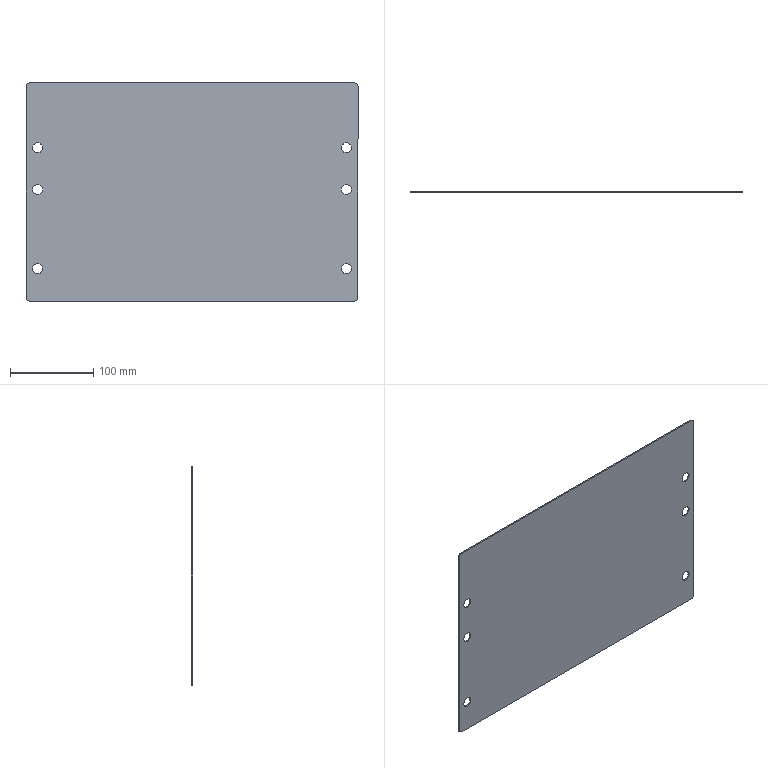Part | SolidWorks | features Fillet 1, FlatPattern 1, HoleWzd 1, SMBaseFlange 1, SheetMetal 1 | 1 solid | 22 faces | box 398 x 1.5 x 262 mm | volume 155364 mm3 | cylinder 16 | plane 6 | commonest cylinder face diameters 12 x12 10 x4
STEP:
#1=CARTESIAN_POINT('',(-185.,-1.5,-3.));
#2=VERTEX_POINT('',#1);
#3=CARTESIAN_POINT('',(-185.,-1.5,9.));
#4=VERTEX_POINT('',#3);
#5=CARTESIAN_POINT('',(-185.,-1.5,3.));
#6=DIRECTION('',(0.,1.,0.));
#7=DIRECTION('',(0.,0.,1.));
#8=AXIS2_PLACEMENT_3D('',#5,#6,#7);
#9=CIRCLE('',#8,6.);
#10=EDGE_CURVE('',#2,#4,#9,.T.);
#11=ORIENTED_EDGE('',*,*,#10,.F.);
#12=CARTESIAN_POINT('',(-185.,0.,-3.));
#13=VERTEX_POINT('',#12);
#14=CARTESIAN_POINT('',(-185.,0.,-3.));
#15=DIRECTION('',(0.,1.,0.));
#16=VECTOR('',#15,1000.);
#17=LINE('',#14,#16);
#18=EDGE_CURVE('',#2,#13,#17,.T.);
#19=ORIENTED_EDGE('',*,*,#18,.T.);
#20=CARTESIAN_POINT('',(-185.,0.,9.));
#21=VERTEX_POINT('',#20);
#22=CARTESIAN_POINT('',(-185.,0.,3.));
#23=DIRECTION('',(0.,1.,0.));
#24=DIRECTION('',(0.,0.,1.));
#25=AXIS2_PLACEMENT_3D('',#22,#23,#24);
#26=CIRCLE('',#25,6.);
#27=EDGE_CURVE('',#13,#21,#26,.T.);
#28=ORIENTED_EDGE('',*,*,#27,.T.);
#29=CARTESIAN_POINT('',(-185.,0.,9.));
#30=DIRECTION('',(0.,1.,0.));
#31=VECTOR('',#30,1000.);
#32=LINE('',#29,#31);
#33=EDGE_CURVE('',#4,#21,#32,.T.);
#34=ORIENTED_EDGE('',*,*,#33,.F.);
#35=EDGE_LOOP('',(#11,#19,#28,#34));
#36=FACE_OUTER_BOUND('',#35,.T.);
#37=CARTESIAN_POINT('',(-185.,0.,3.));
#38=DIRECTION('',(0.,1.,0.));
#39=DIRECTION('',(0.,0.,1.));
#40=AXIS2_PLACEMENT_3D('',#37,#38,#39);
#41=CYLINDRICAL_SURFACE('',#40,6.);
#42=ADVANCED_FACE('',(#36),#41,.F.);
#43=CARTESIAN_POINT('',(-185.,-1.5,47.));
#44=VERTEX_POINT('',#43);
#45=CARTESIAN_POINT('',(-185.,-1.5,59.));
#46=VERTEX_POINT('',#45);
#47=CARTESIAN_POINT('',(-185.,-1.5,53.));
#48=DIRECTION('',(0.,1.,0.));
#49=DIRECTION('',(0.,0.,1.));
#50=AXIS2_PLACEMENT_3D('',#47,#48,#49);
#51=CIRCLE('',#50,6.);
#52=EDGE_CURVE('',#44,#46,#51,.T.);
#53=ORIENTED_EDGE('',*,*,#52,.F.);
#54=CARTESIAN_POINT('',(-185.,0.,47.));
#55=VERTEX_POINT('',#54);
#56=CARTESIAN_POINT('',(-185.,0.,47.));
#57=DIRECTION('',(0.,1.,0.));
#58=VECTOR('',#57,1000.);
#59=LINE('',#56,#58);
#60=EDGE_CURVE('',#44,#55,#59,.T.);
#61=ORIENTED_EDGE('',*,*,#60,.T.);
#62=CARTESIAN_POINT('',(-185.,0.,59.));
#63=VERTEX_POINT('',#62);
#64=CARTESIAN_POINT('',(-185.,0.,53.));
#65=DIRECTION('',(0.,1.,0.));
#66=DIRECTION('',(0.,0.,1.));
#67=AXIS2_PLACEMENT_3D('',#64,#65,#66);
#68=CIRCLE('',#67,6.);
#69=EDGE_CURVE('',#55,#63,#68,.T.);
#70=ORIENTED_EDGE('',*,*,#69,.T.);
#71=CARTESIAN_POINT('',(-185.,0.,59.));
#72=DIRECTION('',(0.,1.,0.));
#73=VECTOR('',#72,1000.);
#74=LINE('',#71,#73);
#75=EDGE_CURVE('',#46,#63,#74,.T.);
#76=ORIENTED_EDGE('',*,*,#75,.F.);
#77=EDGE_LOOP('',(#53,#61,#70,#76));
#78=FACE_OUTER_BOUND('',#77,.T.);
#79=CARTESIAN_POINT('',(-185.,0.,53.));
#80=DIRECTION('',(0.,1.,0.));
#81=DIRECTION('',(0.,0.,1.));
#82=AXIS2_PLACEMENT_3D('',#79,#80,#81);
#83=CYLINDRICAL_SURFACE('',#82,6.);
#84=ADVANCED_FACE('',(#78),#83,.F.);
#85=CARTESIAN_POINT('',(185.,-1.5,-3.));
#86=VERTEX_POINT('',#85);
#87=CARTESIAN_POINT('',(185.,-1.5,9.));
#88=VERTEX_POINT('',#87);
#89=CARTESIAN_POINT('',(185.,-1.5,3.));
#90=DIRECTION('',(0.,1.,0.));
#91=DIRECTION('',(0.,0.,1.));
#92=AXIS2_PLACEMENT_3D('',#89,#90,#91);
#93=CIRCLE('',#92,6.);
#94=EDGE_CURVE('',#86,#88,#93,.T.);
#95=ORIENTED_EDGE('',*,*,#94,.F.);
#96=CARTESIAN_POINT('',(185.,0.,-3.));
#97=VERTEX_POINT('',#96);
#98=CARTESIAN_POINT('',(185.,0.,-3.));
#99=DIRECTION('',(0.,1.,0.));
#100=VECTOR('',#99,1000.);
#101=LINE('',#98,#100);
#102=EDGE_CURVE('',#86,#97,#101,.T.);
#103=ORIENTED_EDGE('',*,*,#102,.T.);
#104=CARTESIAN_POINT('',(185.,0.,9.));
#105=VERTEX_POINT('',#104);
#106=CARTESIAN_POINT('',(185.,0.,3.));
#107=DIRECTION('',(0.,1.,0.));
#108=DIRECTION('',(0.,0.,1.));
#109=AXIS2_PLACEMENT_3D('',#106,#107,#108);
#110=CIRCLE('',#109,6.);
#111=EDGE_CURVE('',#97,#105,#110,.T.);
#112=ORIENTED_EDGE('',*,*,#111,.T.);
#113=CARTESIAN_POINT('',(185.,0.,9.));
#114=DIRECTION('',(0.,1.,0.));
#115=VECTOR('',#114,1000.);
#116=LINE('',#113,#115);
#117=EDGE_CURVE('',#88,#105,#116,.T.);
#118=ORIENTED_EDGE('',*,*,#117,.F.);
#119=EDGE_LOOP('',(#95,#103,#112,#118));
#120=FACE_OUTER_BOUND('',#119,.T.);
#121=CARTESIAN_POINT('',(185.,0.,3.));
#122=DIRECTION('',(0.,1.,0.));
#123=DIRECTION('',(0.,0.,1.));
#124=AXIS2_PLACEMENT_3D('',#121,#122,#123);
#125=CYLINDRICAL_SURFACE('',#124,6.);
#126=ADVANCED_FACE('',(#120),#125,.F.);
#127=CARTESIAN_POINT('',(185.,-1.5,47.));
#128=VERTEX_POINT('',#127);
#129=CARTESIAN_POINT('',(185.,-1.5,59.));
#130=VERTEX_POINT('',#129);
#131=CARTESIAN_POINT('',(185.,-1.5,53.));
#132=DIRECTION('',(0.,1.,0.));
#133=DIRECTION('',(0.,0.,1.));
#134=AXIS2_PLACEMENT_3D('',#131,#132,#133);
#135=CIRCLE('',#134,6.);
#136=EDGE_CURVE('',#128,#130,#135,.T.);
#137=ORIENTED_EDGE('',*,*,#136,.F.);
#138=CARTESIAN_POINT('',(185.,0.,47.));
#139=VERTEX_POINT('',#138);
#140=CARTESIAN_POINT('',(185.,0.,47.));
#141=DIRECTION('',(0.,1.,0.));
#142=VECTOR('',#141,1000.);
#143=LINE('',#140,#142);
#144=EDGE_CURVE('',#128,#139,#143,.T.);
#145=ORIENTED_EDGE('',*,*,#144,.T.);
#146=CARTESIAN_POINT('',(185.,0.,59.));
#147=VERTEX_POINT('',#146);
#148=CARTESIAN_POINT('',(185.,0.,53.));
#149=DIRECTION('',(0.,1.,0.));
#150=DIRECTION('',(0.,0.,1.));
#151=AXIS2_PLACEMENT_3D('',#148,#149,#150);
#152=CIRCLE('',#151,6.);
#153=EDGE_CURVE('',#139,#147,#152,.T.);
#154=ORIENTED_EDGE('',*,*,#153,.T.);
#155=CARTESIAN_POINT('',(185.,0.,59.));
#156=DIRECTION('',(0.,1.,0.));
#157=VECTOR('',#156,1000.);
#158=LINE('',#155,#157);
#159=EDGE_CURVE('',#130,#147,#158,.T.);
#160=ORIENTED_EDGE('',*,*,#159,.F.);
#161=EDGE_LOOP('',(#137,#145,#154,#160));
#162=FACE_OUTER_BOUND('',#161,.T.);
#163=CARTESIAN_POINT('',(185.,0.,53.));
#164=DIRECTION('',(0.,1.,0.));
#165=DIRECTION('',(0.,0.,1.));
#166=AXIS2_PLACEMENT_3D('',#163,#164,#165);
#167=CYLINDRICAL_SURFACE('',#166,6.);
#168=ADVANCED_FACE('',(#162),#167,.F.);
#169=CARTESIAN_POINT('',(-185.,-1.5,-98.));
#170=VERTEX_POINT('',#169);
#171=CARTESIAN_POINT('',(-185.,-1.5,-86.));
#172=VERTEX_POINT('',#171);
#173=CARTESIAN_POINT('',(-185.,-1.5,-92.));
#174=DIRECTION('',(0.,1.,0.));
#175=DIRECTION('',(0.,0.,1.));
#176=AXIS2_PLACEMENT_3D('',#173,#174,#175);
#177=CIRCLE('',#176,6.);
#178=EDGE_CURVE('',#170,#172,#177,.T.);
#179=ORIENTED_EDGE('',*,*,#178,.F.);
#180=CARTESIAN_POINT('',(-185.,0.,-98.));
#181=VERTEX_POINT('',#180);
#182=CARTESIAN_POINT('',(-185.,0.,-98.));
#183=DIRECTION('',(0.,1.,0.));
#184=VECTOR('',#183,1000.);
#185=LINE('',#182,#184);
#186=EDGE_CURVE('',#170,#181,#185,.T.);
#187=ORIENTED_EDGE('',*,*,#186,.T.);
#188=CARTESIAN_POINT('',(-185.,0.,-86.));
#189=VERTEX_POINT('',#188);
#190=CARTESIAN_POINT('',(-185.,0.,-92.));
#191=DIRECTION('',(0.,1.,0.));
#192=DIRECTION('',(0.,0.,1.));
#193=AXIS2_PLACEMENT_3D('',#190,#191,#192);
#194=CIRCLE('',#193,6.);
#195=EDGE_CURVE('',#181,#189,#194,.T.);
#196=ORIENTED_EDGE('',*,*,#195,.T.);
#197=CARTESIAN_POINT('',(-185.,0.,-86.));
#198=DIRECTION('',(0.,1.,0.));
#199=VECTOR('',#198,1000.);
#200=LINE('',#197,#199);
#201=EDGE_CURVE('',#172,#189,#200,.T.);
#202=ORIENTED_EDGE('',*,*,#201,.F.);
#203=EDGE_LOOP('',(#179,#187,#196,#202));
#204=FACE_OUTER_BOUND('',#203,.T.);
#205=CARTESIAN_POINT('',(-185.,0.,-92.));
#206=DIRECTION('',(0.,1.,0.));
#207=DIRECTION('',(0.,0.,1.));
#208=AXIS2_PLACEMENT_3D('',#205,#206,#207);
#209=CYLINDRICAL_SURFACE('',#208,6.);
#210=ADVANCED_FACE('',(#204),#209,.F.);
#211=CARTESIAN_POINT('',(185.,-1.5,-98.));
#212=VERTEX_POINT('',#211);
#213=CARTESIAN_POINT('',(185.,-1.5,-86.));
#214=VERTEX_POINT('',#213);
#215=CARTESIAN_POINT('',(185.,-1.5,-92.));
#216=DIRECTION('',(0.,1.,0.));
#217=DIRECTION('',(0.,0.,1.));
#218=AXIS2_PLACEMENT_3D('',#215,#216,#217);
#219=CIRCLE('',#218,6.);
#220=EDGE_CURVE('',#212,#214,#219,.T.);
#221=ORIENTED_EDGE('',*,*,#220,.F.);
#222=CARTESIAN_POINT('',(185.,0.,-98.));
#223=VERTEX_POINT('',#222);
#224=CARTESIAN_POINT('',(185.,0.,-98.));
#225=DIRECTION('',(0.,1.,0.));
#226=VECTOR('',#225,1000.);
#227=LINE('',#224,#226);
#228=EDGE_CURVE('',#212,#223,#227,.T.);
#229=ORIENTED_EDGE('',*,*,#228,.T.);
#230=CARTESIAN_POINT('',(185.,0.,-86.));
#231=VERTEX_POINT('',#230);
#232=CARTESIAN_POINT('',(185.,0.,-92.));
#233=DIRECTION('',(0.,1.,0.));
#234=DIRECTION('',(0.,0.,1.));
#235=AXIS2_PLACEMENT_3D('',#232,#233,#234);
#236=CIRCLE('',#235,6.);
#237=EDGE_CURVE('',#223,#231,#236,.T.);
#238=ORIENTED_EDGE('',*,*,#237,.T.);
#239=CARTESIAN_POINT('',(185.,0.,-86.));
#240=DIRECTION('',(0.,1.,0.));
#241=VECTOR('',#240,1000.);
#242=LINE('',#239,#241);
#243=EDGE_CURVE('',#214,#231,#242,.T.);
#244=ORIENTED_EDGE('',*,*,#243,.F.);
#245=EDGE_LOOP('',(#221,#229,#238,#244));
#246=FACE_OUTER_BOUND('',#245,.T.);
#247=CARTESIAN_POINT('',(185.,0.,-92.));
#248=DIRECTION('',(0.,1.,0.));
#249=DIRECTION('',(0.,0.,1.));
#250=AXIS2_PLACEMENT_3D('',#247,#248,#249);
#251=CYLINDRICAL_SURFACE('',#250,6.);
#252=ADVANCED_FACE('',(#246),#251,.F.);
#253=CARTESIAN_POINT('',(199.,-1.5,126.));
#254=VERTEX_POINT('',#253);
#255=CARTESIAN_POINT('',(199.,-1.5,-126.));
#256=VERTEX_POINT('',#255);
#257=CARTESIAN_POINT('',(199.,-1.5,-131.));
#258=DIRECTION('',(0.,0.,-1.));
#259=VECTOR('',#258,1000.);
#260=LINE('',#257,#259);
#261=EDGE_CURVE('',#254,#256,#260,.T.);
#262=ORIENTED_EDGE('',*,*,#261,.T.);
#263=CARTESIAN_POINT('',(199.,0.,-126.));
#264=VERTEX_POINT('',#263);
#265=CARTESIAN_POINT('',(199.,-1.5,-126.));
#266=DIRECTION('',(0.,1.,0.));
#267=VECTOR('',#266,1000.);
#268=LINE('',#265,#267);
#269=EDGE_CURVE('',#256,#264,#268,.T.);
#270=ORIENTED_EDGE('',*,*,#269,.T.);
#271=CARTESIAN_POINT('',(199.,0.,126.));
#272=VERTEX_POINT('',#271);
#273=CARTESIAN_POINT('',(199.,0.,-131.));
#274=DIRECTION('',(0.,0.,-1.));
#275=VECTOR('',#274,1000.);
#276=LINE('',#273,#275);
#277=EDGE_CURVE('',#272,#264,#276,.T.);
#278=ORIENTED_EDGE('',*,*,#277,.F.);
#279=CARTESIAN_POINT('',(199.,-1.5,126.));
#280=DIRECTION('',(0.,-1.,0.));
#281=VECTOR('',#280,1000.);
#282=LINE('',#279,#281);
#283=EDGE_CURVE('',#272,#254,#282,.T.);
#284=ORIENTED_EDGE('',*,*,#283,.T.);
#285=EDGE_LOOP('',(#262,#270,#278,#284));
#286=FACE_OUTER_BOUND('',#285,.T.);
#287=CARTESIAN_POINT('',(199.,-1.5,-131.));
#288=DIRECTION('',(1.,0.,0.));
#289=DIRECTION('',(0.,0.,-1.));
#290=AXIS2_PLACEMENT_3D('',#287,#288,#289);
#291=PLANE('',#290);
#292=ADVANCED_FACE('',(#286),#291,.T.);
#293=CARTESIAN_POINT('',(-194.,-1.5,131.));
#294=VERTEX_POINT('',#293);
#295=CARTESIAN_POINT('',(194.,-1.5,131.));
#296=VERTEX_POINT('',#295);
#297=CARTESIAN_POINT('',(-199.,-1.5,131.));
#298=DIRECTION('',(1.,0.,0.));
#299=VECTOR('',#298,1000.);
#300=LINE('',#297,#299);
#301=EDGE_CURVE('',#294,#296,#300,.T.);
#302=ORIENTED_EDGE('',*,*,#301,.T.);
#303=CARTESIAN_POINT('',(194.,0.,131.));
#304=VERTEX_POINT('',#303);
#305=CARTESIAN_POINT('',(194.,-1.5,131.));
#306=DIRECTION('',(0.,1.,0.));
#307=VECTOR('',#306,1000.);
#308=LINE('',#305,#307);
#309=EDGE_CURVE('',#296,#304,#308,.T.);
#310=ORIENTED_EDGE('',*,*,#309,.T.);
#311=CARTESIAN_POINT('',(-194.,0.,131.));
#312=VERTEX_POINT('',#311);
#313=CARTESIAN_POINT('',(-199.,0.,131.));
#314=DIRECTION('',(1.,0.,0.));
#315=VECTOR('',#314,1000.);
#316=LINE('',#313,#315);
#317=EDGE_CURVE('',#312,#304,#316,.T.);
#318=ORIENTED_EDGE('',*,*,#317,.F.);
#319=CARTESIAN_POINT('',(-194.,-1.5,131.));
#320=DIRECTION('',(0.,-1.,0.));
#321=VECTOR('',#320,1000.);
#322=LINE('',#319,#321);
#323=EDGE_CURVE('',#312,#294,#322,.T.);
#324=ORIENTED_EDGE('',*,*,#323,.T.);
#325=EDGE_LOOP('',(#302,#310,#318,#324));
#326=FACE_OUTER_BOUND('',#325,.T.);
#327=CARTESIAN_POINT('',(-199.,-1.5,131.));
#328=DIRECTION('',(0.,0.,1.));
#329=DIRECTION('',(1.,0.,0.));
#330=AXIS2_PLACEMENT_3D('',#327,#328,#329);
#331=PLANE('',#330);
#332=ADVANCED_FACE('',(#326),#331,.T.);
#333=CARTESIAN_POINT('',(-199.,0.,-126.));
#334=VERTEX_POINT('',#333);
#335=CARTESIAN_POINT('',(-199.,0.,126.));
#336=VERTEX_POINT('',#335);
#337=CARTESIAN_POINT('',(-199.,0.,-131.));
#338=DIRECTION('',(0.,0.,1.));
#339=VECTOR('',#338,1000.);
#340=LINE('',#337,#339);
#341=EDGE_CURVE('',#334,#336,#340,.T.);
#342=ORIENTED_EDGE('',*,*,#341,.F.);
#343=CARTESIAN_POINT('',(-199.,-1.5,-126.));
#344=VERTEX_POINT('',#343);
#345=CARTESIAN_POINT('',(-199.,-1.5,-126.));
#346=DIRECTION('',(0.,-1.,0.));
#347=VECTOR('',#346,1000.);
#348=LINE('',#345,#347);
#349=EDGE_CURVE('',#334,#344,#348,.T.);
#350=ORIENTED_EDGE('',*,*,#349,.T.);
#351=CARTESIAN_POINT('',(-199.,-1.5,126.));
#352=VERTEX_POINT('',#351);
#353=CARTESIAN_POINT('',(-199.,-1.5,-131.));
#354=DIRECTION('',(0.,0.,1.));
#355=VECTOR('',#354,1000.);
#356=LINE('',#353,#355);
#357=EDGE_CURVE('',#344,#352,#356,.T.);
#358=ORIENTED_EDGE('',*,*,#357,.T.);
#359=CARTESIAN_POINT('',(-199.,-1.5,126.));
#360=DIRECTION('',(0.,1.,0.));
#361=VECTOR('',#360,1000.);
#362=LINE('',#359,#361);
#363=EDGE_CURVE('',#352,#336,#362,.T.);
#364=ORIENTED_EDGE('',*,*,#363,.T.);
#365=EDGE_LOOP('',(#342,#350,#358,#364));
#366=FACE_OUTER_BOUND('',#365,.T.);
#367=CARTESIAN_POINT('',(-199.,-1.5,-131.));
#368=DIRECTION('',(-1.,0.,0.));
#369=DIRECTION('',(0.,0.,1.));
#370=AXIS2_PLACEMENT_3D('',#367,#368,#369);
#371=PLANE('',#370);
#372=ADVANCED_FACE('',(#366),#371,.T.);
#373=CARTESIAN_POINT('',(194.,-1.5,-131.));
#374=VERTEX_POINT('',#373);
#375=CARTESIAN_POINT('',(-194.,-1.5,-131.));
#376=VERTEX_POINT('',#375);
#377=CARTESIAN_POINT('',(-199.,-1.5,-131.));
#378=DIRECTION('',(-1.,0.,0.));
#379=VECTOR('',#378,1000.);
#380=LINE('',#377,#379);
#381=EDGE_CURVE('',#374,#376,#380,.T.);
#382=ORIENTED_EDGE('',*,*,#381,.T.);
#383=CARTESIAN_POINT('',(-194.,0.,-131.));
#384=VERTEX_POINT('',#383);
#385=CARTESIAN_POINT('',(-194.,-1.5,-131.));
#386=DIRECTION('',(0.,1.,0.));
#387=VECTOR('',#386,1000.);
#388=LINE('',#385,#387);
#389=EDGE_CURVE('',#376,#384,#388,.T.);
#390=ORIENTED_EDGE('',*,*,#389,.T.);
#391=CARTESIAN_POINT('',(194.,0.,-131.));
#392=VERTEX_POINT('',#391);
#393=CARTESIAN_POINT('',(-199.,0.,-131.));
#394=DIRECTION('',(-1.,0.,0.));
#395=VECTOR('',#394,1000.);
#396=LINE('',#393,#395);
#397=EDGE_CURVE('',#392,#384,#396,.T.);
#398=ORIENTED_EDGE('',*,*,#397,.F.);
#399=CARTESIAN_POINT('',(194.,-1.5,-131.));
#400=DIRECTION('',(0.,-1.,0.));
#401=VECTOR('',#400,1000.);
#402=LINE('',#399,#401);
#403=EDGE_CURVE('',#392,#374,#402,.T.);
#404=ORIENTED_EDGE('',*,*,#403,.T.);
#405=EDGE_LOOP('',(#382,#390,#398,#404));
#406=FACE_OUTER_BOUND('',#405,.T.);
#407=CARTESIAN_POINT('',(-199.,-1.5,-131.));
#408=DIRECTION('',(0.,0.,-1.));
#409=DIRECTION('',(-1.,0.,0.));
#410=AXIS2_PLACEMENT_3D('',#407,#408,#409);
#411=PLANE('',#410);
#412=ADVANCED_FACE('',(#406),#411,.T.);
#413=CARTESIAN_POINT('',(-185.,-1.5,3.));
#414=DIRECTION('',(0.,1.,0.));
#415=DIRECTION('',(0.,0.,1.));
#416=AXIS2_PLACEMENT_3D('',#413,#414,#415);
#417=CIRCLE('',#416,6.);
#418=EDGE_CURVE('',#4,#2,#417,.T.);
#419=ORIENTED_EDGE('',*,*,#418,.T.);
#420=ORIENTED_EDGE('',*,*,#10,.T.);
#421=EDGE_LOOP('',(#419,#420));
#422=FACE_BOUND('',#421,.T.);
#423=CARTESIAN_POINT('',(-185.,-1.5,53.));
#424=DIRECTION('',(0.,1.,0.));
#425=DIRECTION('',(0.,0.,1.));
#426=AXIS2_PLACEMENT_3D('',#423,#424,#425);
#427=CIRCLE('',#426,6.);
#428=EDGE_CURVE('',#46,#44,#427,.T.);
#429=ORIENTED_EDGE('',*,*,#428,.T.);
#430=ORIENTED_EDGE('',*,*,#52,.T.);
#431=EDGE_LOOP('',(#429,#430));
#432=FACE_BOUND('',#431,.T.);
#433=CARTESIAN_POINT('',(185.,-1.5,3.));
#434=DIRECTION('',(0.,1.,0.));
#435=DIRECTION('',(0.,0.,1.));
#436=AXIS2_PLACEMENT_3D('',#433,#434,#435);
#437=CIRCLE('',#436,6.);
#438=EDGE_CURVE('',#88,#86,#437,.T.);
#439=ORIENTED_EDGE('',*,*,#438,.T.);
#440=ORIENTED_EDGE('',*,*,#94,.T.);
#441=EDGE_LOOP('',(#439,#440));
#442=FACE_BOUND('',#441,.T.);
#443=CARTESIAN_POINT('',(185.,-1.5,53.));
#444=DIRECTION('',(0.,1.,0.));
#445=DIRECTION('',(0.,0.,1.));
#446=AXIS2_PLACEMENT_3D('',#443,#444,#445);
#447=CIRCLE('',#446,6.);
#448=EDGE_CURVE('',#130,#128,#447,.T.);
#449=ORIENTED_EDGE('',*,*,#448,.T.);
#450=ORIENTED_EDGE('',*,*,#136,.T.);
#451=EDGE_LOOP('',(#449,#450));
#452=FACE_BOUND('',#451,.T.);
#453=CARTESIAN_POINT('',(-185.,-1.5,-92.));
#454=DIRECTION('',(0.,1.,0.));
#455=DIRECTION('',(0.,0.,1.));
#456=AXIS2_PLACEMENT_3D('',#453,#454,#455);
#457=CIRCLE('',#456,6.);
#458=EDGE_CURVE('',#172,#170,#457,.T.);
#459=ORIENTED_EDGE('',*,*,#458,.T.);
#460=ORIENTED_EDGE('',*,*,#178,.T.);
#461=EDGE_LOOP('',(#459,#460));
#462=FACE_BOUND('',#461,.T.);
#463=CARTESIAN_POINT('',(185.,-1.5,-92.));
#464=DIRECTION('',(0.,1.,0.));
#465=DIRECTION('',(0.,0.,1.));
#466=AXIS2_PLACEMENT_3D('',#463,#464,#465);
#467=CIRCLE('',#466,6.);
#468=EDGE_CURVE('',#214,#212,#467,.T.);
#469=ORIENTED_EDGE('',*,*,#468,.T.);
#470=ORIENTED_EDGE('',*,*,#220,.T.);
#471=EDGE_LOOP('',(#469,#470));
#472=FACE_BOUND('',#471,.T.);
#473=ORIENTED_EDGE('',*,*,#357,.F.);
#474=CARTESIAN_POINT('',(-194.,-1.5,-126.));
#475=DIRECTION('',(0.,-1.,0.));
#476=DIRECTION('',(0.,0.,1.));
#477=AXIS2_PLACEMENT_3D('',#474,#475,#476);
#478=CIRCLE('',#477,5.);
#479=EDGE_CURVE('',#344,#376,#478,.T.);
#480=ORIENTED_EDGE('',*,*,#479,.T.);
#481=ORIENTED_EDGE('',*,*,#381,.F.);
#482=CARTESIAN_POINT('',(194.,-1.5,-126.));
#483=DIRECTION('',(0.,-1.,0.));
#484=DIRECTION('',(0.,0.,1.));
#485=AXIS2_PLACEMENT_3D('',#482,#483,#484);
#486=CIRCLE('',#485,5.);
#487=EDGE_CURVE('',#374,#256,#486,.T.);
#488=ORIENTED_EDGE('',*,*,#487,.T.);
#489=ORIENTED_EDGE('',*,*,#261,.F.);
#490=CARTESIAN_POINT('',(194.,-1.5,126.));
#491=DIRECTION('',(0.,-1.,0.));
#492=DIRECTION('',(0.,0.,1.));
#493=AXIS2_PLACEMENT_3D('',#490,#491,#492);
#494=CIRCLE('',#493,5.);
#495=EDGE_CURVE('',#254,#296,#494,.T.);
#496=ORIENTED_EDGE('',*,*,#495,.T.);
#497=ORIENTED_EDGE('',*,*,#301,.F.);
#498=CARTESIAN_POINT('',(-194.,-1.5,126.));
#499=DIRECTION('',(0.,-1.,0.));
#500=DIRECTION('',(0.,0.,1.));
#501=AXIS2_PLACEMENT_3D('',#498,#499,#500);
#502=CIRCLE('',#501,5.);
#503=EDGE_CURVE('',#294,#352,#502,.T.);
#504=ORIENTED_EDGE('',*,*,#503,.T.);
#505=EDGE_LOOP('',(#473,#480,#481,#488,#489,#496,#497,#504));
#506=FACE_OUTER_BOUND('',#505,.T.);
#507=CARTESIAN_POINT('',(0.,-1.5,0.));
#508=DIRECTION('',(0.,1.,0.));
#509=DIRECTION('',(0.,0.,1.));
#510=AXIS2_PLACEMENT_3D('',#507,#508,#509);
#511=PLANE('',#510);
#512=ADVANCED_FACE('',(#422,#432,#442,#452,#462,#472,#506),#511,.F.);
#513=CARTESIAN_POINT('',(-185.,0.,3.));
#514=DIRECTION('',(0.,1.,0.));
#515=DIRECTION('',(0.,0.,1.));
#516=AXIS2_PLACEMENT_3D('',#513,#514,#515);
#517=CIRCLE('',#516,6.);
#518=EDGE_CURVE('',#21,#13,#517,.T.);
#519=ORIENTED_EDGE('',*,*,#518,.F.);
#520=ORIENTED_EDGE('',*,*,#27,.F.);
#521=EDGE_LOOP('',(#519,#520));
#522=FACE_BOUND('',#521,.T.);
#523=CARTESIAN_POINT('',(-185.,0.,53.));
#524=DIRECTION('',(0.,1.,0.));
#525=DIRECTION('',(0.,0.,1.));
#526=AXIS2_PLACEMENT_3D('',#523,#524,#525);
#527=CIRCLE('',#526,6.);
#528=EDGE_CURVE('',#63,#55,#527,.T.);
#529=ORIENTED_EDGE('',*,*,#528,.F.);
#530=ORIENTED_EDGE('',*,*,#69,.F.);
#531=EDGE_LOOP('',(#529,#530));
#532=FACE_BOUND('',#531,.T.);
#533=CARTESIAN_POINT('',(185.,0.,3.));
#534=DIRECTION('',(0.,1.,0.));
#535=DIRECTION('',(0.,0.,1.));
#536=AXIS2_PLACEMENT_3D('',#533,#534,#535);
#537=CIRCLE('',#536,6.);
#538=EDGE_CURVE('',#105,#97,#537,.T.);
#539=ORIENTED_EDGE('',*,*,#538,.F.);
#540=ORIENTED_EDGE('',*,*,#111,.F.);
#541=EDGE_LOOP('',(#539,#540));
#542=FACE_BOUND('',#541,.T.);
#543=CARTESIAN_POINT('',(185.,0.,53.));
#544=DIRECTION('',(0.,1.,0.));
#545=DIRECTION('',(0.,0.,1.));
#546=AXIS2_PLACEMENT_3D('',#543,#544,#545);
#547=CIRCLE('',#546,6.);
#548=EDGE_CURVE('',#147,#139,#547,.T.);
#549=ORIENTED_EDGE('',*,*,#548,.F.);
#550=ORIENTED_EDGE('',*,*,#153,.F.);
#551=EDGE_LOOP('',(#549,#550));
#552=FACE_BOUND('',#551,.T.);
#553=CARTESIAN_POINT('',(-185.,0.,-92.));
#554=DIRECTION('',(0.,1.,0.));
#555=DIRECTION('',(0.,0.,1.));
#556=AXIS2_PLACEMENT_3D('',#553,#554,#555);
#557=CIRCLE('',#556,6.);
#558=EDGE_CURVE('',#189,#181,#557,.T.);
#559=ORIENTED_EDGE('',*,*,#558,.F.);
#560=ORIENTED_EDGE('',*,*,#195,.F.);
#561=EDGE_LOOP('',(#559,#560));
#562=FACE_BOUND('',#561,.T.);
#563=CARTESIAN_POINT('',(185.,0.,-92.));
#564=DIRECTION('',(0.,1.,0.));
#565=DIRECTION('',(0.,0.,1.));
#566=AXIS2_PLACEMENT_3D('',#563,#564,#565);
#567=CIRCLE('',#566,6.);
#568=EDGE_CURVE('',#231,#223,#567,.T.);
#569=ORIENTED_EDGE('',*,*,#568,.F.);
#570=ORIENTED_EDGE('',*,*,#237,.F.);
#571=EDGE_LOOP('',(#569,#570));
#572=FACE_BOUND('',#571,.T.);
#573=ORIENTED_EDGE('',*,*,#397,.T.);
#574=CARTESIAN_POINT('',(-194.,0.,-126.));
#575=DIRECTION('',(0.,1.,0.));
#576=DIRECTION('',(0.,0.,1.));
#577=AXIS2_PLACEMENT_3D('',#574,#575,#576);
#578=CIRCLE('',#577,5.);
#579=EDGE_CURVE('',#384,#334,#578,.T.);
#580=ORIENTED_EDGE('',*,*,#579,.T.);
#581=ORIENTED_EDGE('',*,*,#341,.T.);
#582=CARTESIAN_POINT('',(-194.,0.,126.));
#583=DIRECTION('',(0.,1.,0.));
#584=DIRECTION('',(0.,0.,1.));
#585=AXIS2_PLACEMENT_3D('',#582,#583,#584);
#586=CIRCLE('',#585,5.);
#587=EDGE_CURVE('',#336,#312,#586,.T.);
#588=ORIENTED_EDGE('',*,*,#587,.T.);
#589=ORIENTED_EDGE('',*,*,#317,.T.);
#590=CARTESIAN_POINT('',(194.,0.,126.));
#591=DIRECTION('',(0.,1.,0.));
#592=DIRECTION('',(0.,0.,1.));
#593=AXIS2_PLACEMENT_3D('',#590,#591,#592);
#594=CIRCLE('',#593,5.);
#595=EDGE_CURVE('',#304,#272,#594,.T.);
#596=ORIENTED_EDGE('',*,*,#595,.T.);
#597=ORIENTED_EDGE('',*,*,#277,.T.);
#598=CARTESIAN_POINT('',(194.,0.,-126.));
#599=DIRECTION('',(0.,1.,0.));
#600=DIRECTION('',(0.,0.,1.));
#601=AXIS2_PLACEMENT_3D('',#598,#599,#600);
#602=CIRCLE('',#601,5.);
#603=EDGE_CURVE('',#264,#392,#602,.T.);
#604=ORIENTED_EDGE('',*,*,#603,.T.);
#605=EDGE_LOOP('',(#573,#580,#581,#588,#589,#596,#597,#604));
#606=FACE_OUTER_BOUND('',#605,.T.);
#607=CARTESIAN_POINT('',(0.,0.,0.));
#608=DIRECTION('',(0.,1.,0.));
#609=DIRECTION('',(0.,0.,1.));
#610=AXIS2_PLACEMENT_3D('',#607,#608,#609);
#611=PLANE('',#610);
#612=ADVANCED_FACE('',(#522,#532,#542,#552,#562,#572,#606),#611,.T.);
#613=ORIENTED_EDGE('',*,*,#228,.F.);
#614=ORIENTED_EDGE('',*,*,#468,.F.);
#615=ORIENTED_EDGE('',*,*,#243,.T.);
#616=ORIENTED_EDGE('',*,*,#568,.T.);
#617=EDGE_LOOP('',(#613,#614,#615,#616));
#618=FACE_OUTER_BOUND('',#617,.T.);
#619=CARTESIAN_POINT('',(185.,0.,-92.));
#620=DIRECTION('',(0.,1.,0.));
#621=DIRECTION('',(0.,0.,1.));
#622=AXIS2_PLACEMENT_3D('',#619,#620,#621);
#623=CYLINDRICAL_SURFACE('',#622,6.);
#624=ADVANCED_FACE('',(#618),#623,.F.);
#625=ORIENTED_EDGE('',*,*,#186,.F.);
#626=ORIENTED_EDGE('',*,*,#458,.F.);
#627=ORIENTED_EDGE('',*,*,#201,.T.);
#628=ORIENTED_EDGE('',*,*,#558,.T.);
#629=EDGE_LOOP('',(#625,#626,#627,#628));
#630=FACE_OUTER_BOUND('',#629,.T.);
#631=CARTESIAN_POINT('',(-185.,0.,-92.));
#632=DIRECTION('',(0.,1.,0.));
#633=DIRECTION('',(0.,0.,1.));
#634=AXIS2_PLACEMENT_3D('',#631,#632,#633);
#635=CYLINDRICAL_SURFACE('',#634,6.);
#636=ADVANCED_FACE('',(#630),#635,.F.);
#637=ORIENTED_EDGE('',*,*,#144,.F.);
#638=ORIENTED_EDGE('',*,*,#448,.F.);
#639=ORIENTED_EDGE('',*,*,#159,.T.);
#640=ORIENTED_EDGE('',*,*,#548,.T.);
#641=EDGE_LOOP('',(#637,#638,#639,#640));
#642=FACE_OUTER_BOUND('',#641,.T.);
#643=CARTESIAN_POINT('',(185.,0.,53.));
#644=DIRECTION('',(0.,1.,0.));
#645=DIRECTION('',(0.,0.,1.));
#646=AXIS2_PLACEMENT_3D('',#643,#644,#645);
#647=CYLINDRICAL_SURFACE('',#646,6.);
#648=ADVANCED_FACE('',(#642),#647,.F.);
#649=ORIENTED_EDGE('',*,*,#102,.F.);
#650=ORIENTED_EDGE('',*,*,#438,.F.);
#651=ORIENTED_EDGE('',*,*,#117,.T.);
#652=ORIENTED_EDGE('',*,*,#538,.T.);
#653=EDGE_LOOP('',(#649,#650,#651,#652));
#654=FACE_OUTER_BOUND('',#653,.T.);
#655=CARTESIAN_POINT('',(185.,0.,3.));
#656=DIRECTION('',(0.,1.,0.));
#657=DIRECTION('',(0.,0.,1.));
#658=AXIS2_PLACEMENT_3D('',#655,#656,#657);
#659=CYLINDRICAL_SURFACE('',#658,6.);
#660=ADVANCED_FACE('',(#654),#659,.F.);
#661=ORIENTED_EDGE('',*,*,#60,.F.);
#662=ORIENTED_EDGE('',*,*,#428,.F.);
#663=ORIENTED_EDGE('',*,*,#75,.T.);
#664=ORIENTED_EDGE('',*,*,#528,.T.);
#665=EDGE_LOOP('',(#661,#662,#663,#664));
#666=FACE_OUTER_BOUND('',#665,.T.);
#667=CARTESIAN_POINT('',(-185.,0.,53.));
#668=DIRECTION('',(0.,1.,0.));
#669=DIRECTION('',(0.,0.,1.));
#670=AXIS2_PLACEMENT_3D('',#667,#668,#669);
#671=CYLINDRICAL_SURFACE('',#670,6.);
#672=ADVANCED_FACE('',(#666),#671,.F.);
#673=ORIENTED_EDGE('',*,*,#18,.F.);
#674=ORIENTED_EDGE('',*,*,#418,.F.);
#675=ORIENTED_EDGE('',*,*,#33,.T.);
#676=ORIENTED_EDGE('',*,*,#518,.T.);
#677=EDGE_LOOP('',(#673,#674,#675,#676));
#678=FACE_OUTER_BOUND('',#677,.T.);
#679=CARTESIAN_POINT('',(-185.,0.,3.));
#680=DIRECTION('',(0.,1.,0.));
#681=DIRECTION('',(0.,0.,1.));
#682=AXIS2_PLACEMENT_3D('',#679,#680,#681);
#683=CYLINDRICAL_SURFACE('',#682,6.);
#684=ADVANCED_FACE('',(#678),#683,.F.);
#685=ORIENTED_EDGE('',*,*,#479,.F.);
#686=ORIENTED_EDGE('',*,*,#349,.F.);
#687=ORIENTED_EDGE('',*,*,#579,.F.);
#688=ORIENTED_EDGE('',*,*,#389,.F.);
#689=EDGE_LOOP('',(#685,#686,#687,#688));
#690=FACE_OUTER_BOUND('',#689,.T.);
#691=CARTESIAN_POINT('',(-194.,-1.5,-126.));
#692=DIRECTION('',(0.,1.,0.));
#693=DIRECTION('',(0.,0.,1.));
#694=AXIS2_PLACEMENT_3D('',#691,#692,#693);
#695=CYLINDRICAL_SURFACE('',#694,5.);
#696=ADVANCED_FACE('',(#690),#695,.T.);
#697=ORIENTED_EDGE('',*,*,#487,.F.);
#698=ORIENTED_EDGE('',*,*,#403,.F.);
#699=ORIENTED_EDGE('',*,*,#603,.F.);
#700=ORIENTED_EDGE('',*,*,#269,.F.);
#701=EDGE_LOOP('',(#697,#698,#699,#700));
#702=FACE_OUTER_BOUND('',#701,.T.);
#703=CARTESIAN_POINT('',(194.,-1.5,-126.));
#704=DIRECTION('',(0.,1.,0.));
#705=DIRECTION('',(0.,0.,1.));
#706=AXIS2_PLACEMENT_3D('',#703,#704,#705);
#707=CYLINDRICAL_SURFACE('',#706,5.);
#708=ADVANCED_FACE('',(#702),#707,.T.);
#709=ORIENTED_EDGE('',*,*,#495,.F.);
#710=ORIENTED_EDGE('',*,*,#283,.F.);
#711=ORIENTED_EDGE('',*,*,#595,.F.);
#712=ORIENTED_EDGE('',*,*,#309,.F.);
#713=EDGE_LOOP('',(#709,#710,#711,#712));
#714=FACE_OUTER_BOUND('',#713,.T.);
#715=CARTESIAN_POINT('',(194.,-1.5,126.));
#716=DIRECTION('',(0.,1.,0.));
#717=DIRECTION('',(0.,0.,1.));
#718=AXIS2_PLACEMENT_3D('',#715,#716,#717);
#719=CYLINDRICAL_SURFACE('',#718,5.);
#720=ADVANCED_FACE('',(#714),#719,.T.);
#721=ORIENTED_EDGE('',*,*,#503,.F.);
#722=ORIENTED_EDGE('',*,*,#323,.F.);
#723=ORIENTED_EDGE('',*,*,#587,.F.);
#724=ORIENTED_EDGE('',*,*,#363,.F.);
#725=EDGE_LOOP('',(#721,#722,#723,#724));
#726=FACE_OUTER_BOUND('',#725,.T.);
#727=CARTESIAN_POINT('',(-194.,-1.5,126.));
#728=DIRECTION('',(0.,1.,0.));
#729=DIRECTION('',(0.,0.,1.));
#730=AXIS2_PLACEMENT_3D('',#727,#728,#729);
#731=CYLINDRICAL_SURFACE('',#730,5.);
#732=ADVANCED_FACE('',(#726),#731,.T.);
#733=CLOSED_SHELL('',(#42,#84,#126,#168,#210,#252,#292,#332,#372,#412,#512,#612,#624,#636,#648,#660,#672,#684,#696,#708,#720,#732));
#734=MANIFOLD_SOLID_BREP('',#733);
#735=CARTESIAN_POINT('',(0.,0.,0.));
#736=DIRECTION('',(0.,0.,1.));
#737=DIRECTION('',(1.,0.,0.));
#738=AXIS2_PLACEMENT_3D('',#735,#736,#737);
#739=(LENGTH_UNIT()NAMED_UNIT(*)SI_UNIT(.MILLI.,.METRE.));
#740=UNCERTAINTY_MEASURE_WITH_UNIT(LENGTH_MEASURE(0.00001),#739,'','');
#741=(NAMED_UNIT(*)PLANE_ANGLE_UNIT()SI_UNIT($,.RADIAN.));
#742=(NAMED_UNIT(*)SI_UNIT($,.STERADIAN.)SOLID_ANGLE_UNIT());
#743=(GEOMETRIC_REPRESENTATION_CONTEXT(3)GLOBAL_UNCERTAINTY_ASSIGNED_CONTEXT((#740))GLOBAL_UNIT_ASSIGNED_CONTEXT((#739,#741,#742))REPRESENTATION_CONTEXT('',''));
#744=ADVANCED_BREP_SHAPE_REPRESENTATION('',(#734,#738),#743);